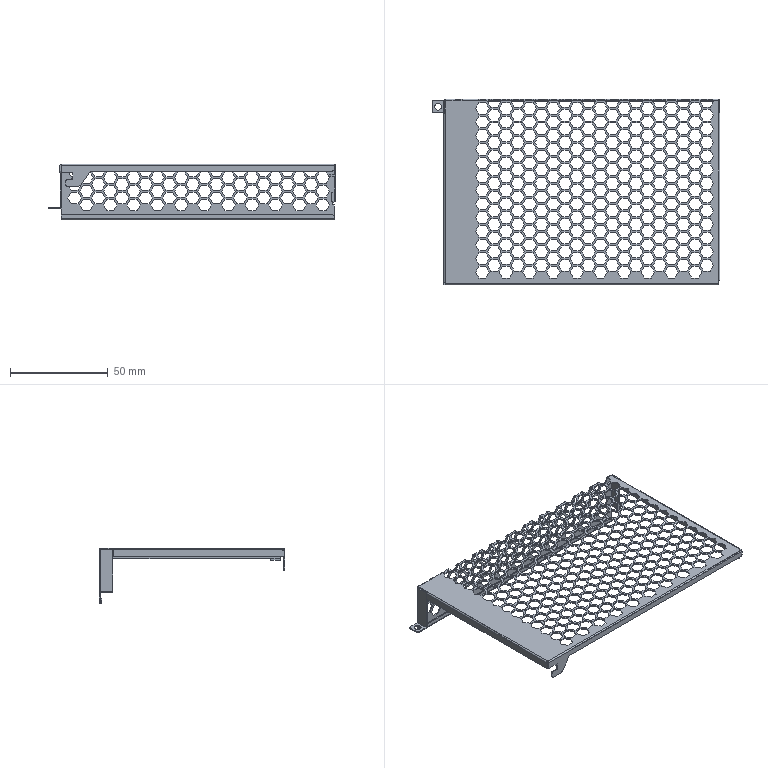Part | STEP file | LRS-150-12_X2_5F00517375-151325 | 1 solid | 2180 faces | box 147.5 x 95.25 x 28.5 mm | volume 5369 mm3 | plane 2071 | cylinder 77 | spline 32 | commonest cylinder face diameters 0.2 x30 1.4 x30 2 x7 1 x4 3.5 x2 0.1 x1